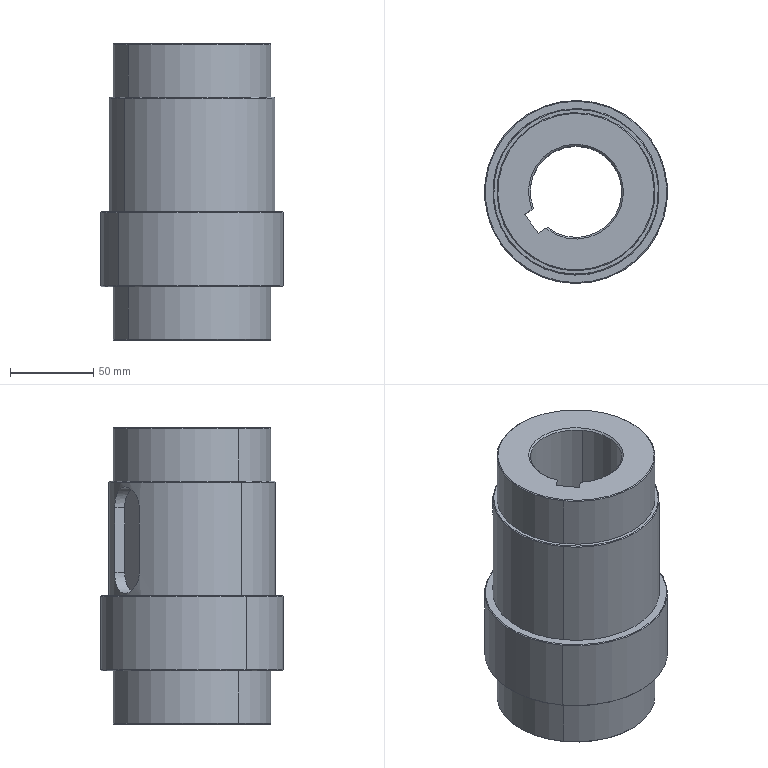Part | SolidWorks | features BaseBody 1 | 1 solid | 37 faces | box 110 x 110 x 178 mm | volume 973022 mm3 | cylinder 13 | cone 13 | plane 11 | commonest cylinder face diameters 95 x4 25 x3 55 x2 100 x2 110 x2
STEP:
#1=CARTESIAN_POINT('',(507.1,275.211,-200.693));
#2=VERTEX_POINT('',#1);
#3=CARTESIAN_POINT('',(497.014,267.828,-188.193));
#4=VERTEX_POINT('',#3);
#5=CARTESIAN_POINT('',(497.014,267.828,-200.693));
#6=DIRECTION('',(0.5907,-0.8069,0.));
#7=DIRECTION('',(0.,0.,-1.));
#8=AXIS2_PLACEMENT_3D('',#5,#6,#7);
#9=CIRCLE('',#8,12.5);
#10=EDGE_CURVE('',#2,#4,#9,.T.);
#11=ORIENTED_EDGE('',*,*,#10,.T.);
#12=CARTESIAN_POINT('',(491.698,275.09,-188.193));
#13=VERTEX_POINT('',#12);
#14=CARTESIAN_POINT('',(497.014,267.828,-188.193));
#15=DIRECTION('',(-0.5907,0.8069,0.));
#16=VECTOR('',#15,1000.);
#17=LINE('',#14,#16);
#18=EDGE_CURVE('',#4,#13,#17,.T.);
#19=ORIENTED_EDGE('',*,*,#18,.T.);
#20=CARTESIAN_POINT('',(502.722,281.192,-200.693));
#21=VERTEX_POINT('',#20);
#22=CARTESIAN_POINT('',(502.722,281.192,-200.693));
#23=CARTESIAN_POINT('',(502.722,281.192,-199.863));
#24=CARTESIAN_POINT('',(502.643,281.161,-199.048));
#25=CARTESIAN_POINT('',(502.414,281.068,-197.846));
#26=CARTESIAN_POINT('',(502.319,281.03,-197.449));
#27=CARTESIAN_POINT('',(502.091,280.936,-196.662));
#28=CARTESIAN_POINT('',(501.958,280.88,-196.272));
#29=CARTESIAN_POINT('',(501.511,280.692,-195.137));
#30=CARTESIAN_POINT('',(501.149,280.536,-194.42));
#31=CARTESIAN_POINT('',(500.514,280.251,-193.403));
#32=CARTESIAN_POINT('',(500.286,280.146,-193.072));
#33=CARTESIAN_POINT('',(499.805,279.922,-192.439));
#34=CARTESIAN_POINT('',(499.554,279.802,-192.137));
#35=CARTESIAN_POINT('',(498.767,279.418,-191.276));
#36=CARTESIAN_POINT('',(498.2,279.13,-190.76));
#37=CARTESIAN_POINT('',(497.289,278.64,-190.075));
#38=CARTESIAN_POINT('',(496.977,278.469,-189.863));
#39=CARTESIAN_POINT('',(496.346,278.113,-189.478));
#40=CARTESIAN_POINT('',(496.025,277.928,-189.304));
#41=CARTESIAN_POINT('',(495.376,277.542,-188.992));
#42=CARTESIAN_POINT('',(495.047,277.342,-188.854));
#43=CARTESIAN_POINT('',(494.38,276.924,-188.615));
#44=CARTESIAN_POINT('',(494.04,276.706,-188.514));
#45=CARTESIAN_POINT('',(493.027,276.038,-188.273));
#46=CARTESIAN_POINT('',(492.359,275.574,-188.193));
#47=CARTESIAN_POINT('',(491.698,275.09,-188.193));
#48=B_SPLINE_CURVE_WITH_KNOTS('',3,(#22,#23,#24,#25,#26,#27,#28,#29,#30,#31,#32,#33,#34,#35,#36,#37,#38,#39,#40,#41,#42,#43,#44,#45,#46,#47),.UNSPECIFIED.,.F.,.F.,(4,2,2,2,2,2,2,2,2,2,2,2,4),(0.,0.002453,0.003679,0.004906,0.007359,0.008585,0.009812,0.01226,0.01349,0.01472,0.01594,0.01717,0.01962),.UNSPECIFIED.);
#49=EDGE_CURVE('',#21,#13,#48,.T.);
#50=ORIENTED_EDGE('',*,*,#49,.F.);
#51=CARTESIAN_POINT('',(507.1,275.211,-200.693));
#52=DIRECTION('',(-0.5907,0.8069,0.));
#53=VECTOR('',#52,1000.);
#54=LINE('',#51,#53);
#55=EDGE_CURVE('',#2,#21,#54,.T.);
#56=ORIENTED_EDGE('',*,*,#55,.F.);
#57=EDGE_LOOP('',(#11,#19,#50,#56));
#58=FACE_OUTER_BOUND('',#57,.T.);
#59=CARTESIAN_POINT('',(497.014,267.828,-200.693));
#60=DIRECTION('',(-0.5907,0.8069,0.));
#61=DIRECTION('',(0.,0.,1.));
#62=AXIS2_PLACEMENT_3D('',#59,#60,#61);
#63=CYLINDRICAL_SURFACE('',#62,12.5);
#64=ADVANCED_FACE('',(#58),#63,.F.);
#65=CARTESIAN_POINT('',(559.156,262.505,-330.693));
#66=VERTEX_POINT('',#65);
#67=CARTESIAN_POINT('',(483.305,206.983,-330.693));
#68=VERTEX_POINT('',#67);
#69=CARTESIAN_POINT('',(521.231,234.744,-330.693));
#70=DIRECTION('',(0.,0.,-1.));
#71=DIRECTION('',(0.8069,0.5907,0.));
#72=AXIS2_PLACEMENT_3D('',#69,#70,#71);
#73=CIRCLE('',#72,47.);
#74=EDGE_CURVE('',#66,#68,#73,.T.);
#75=ORIENTED_EDGE('',*,*,#74,.F.);
#76=CARTESIAN_POINT('',(559.559,262.8,-330.193));
#77=VERTEX_POINT('',#76);
#78=CARTESIAN_POINT('',(559.156,262.505,-330.693));
#79=DIRECTION('',(0.5706,0.4177,0.7071));
#80=VECTOR('',#79,1000.);
#81=LINE('',#78,#80);
#82=EDGE_CURVE('',#66,#77,#81,.T.);
#83=ORIENTED_EDGE('',*,*,#82,.T.);
#84=CARTESIAN_POINT('',(482.902,206.688,-330.193));
#85=VERTEX_POINT('',#84);
#86=CARTESIAN_POINT('',(521.231,234.744,-330.193));
#87=DIRECTION('',(0.,0.,1.));
#88=DIRECTION('',(0.8069,0.5907,0.));
#89=AXIS2_PLACEMENT_3D('',#86,#87,#88);
#90=CIRCLE('',#89,47.5);
#91=EDGE_CURVE('',#85,#77,#90,.T.);
#92=ORIENTED_EDGE('',*,*,#91,.F.);
#93=CARTESIAN_POINT('',(483.305,206.983,-330.693));
#94=DIRECTION('',(-0.5706,-0.4177,0.7071));
#95=VECTOR('',#94,1000.);
#96=LINE('',#93,#95);
#97=EDGE_CURVE('',#68,#85,#96,.T.);
#98=ORIENTED_EDGE('',*,*,#97,.F.);
#99=EDGE_LOOP('',(#75,#83,#92,#98));
#100=FACE_OUTER_BOUND('',#99,.T.);
#101=CARTESIAN_POINT('',(521.231,234.744,-330.693));
#102=DIRECTION('',(0.,0.,1.));
#103=DIRECTION('',(-0.8069,-0.5907,0.));
#104=AXIS2_PLACEMENT_3D('',#101,#102,#103);
#105=CONICAL_SURFACE('',#104,47.,0.7854);
#106=ADVANCED_FACE('',(#100),#105,.T.);
#107=CARTESIAN_POINT('',(565.208,266.935,-298.693));
#108=VERTEX_POINT('',#107);
#109=CARTESIAN_POINT('',(477.253,202.553,-298.693));
#110=VERTEX_POINT('',#109);
#111=CARTESIAN_POINT('',(521.231,234.744,-298.693));
#112=DIRECTION('',(0.,0.,-1.));
#113=DIRECTION('',(0.8069,0.5907,0.));
#114=AXIS2_PLACEMENT_3D('',#111,#112,#113);
#115=CIRCLE('',#114,54.5);
#116=EDGE_CURVE('',#108,#110,#115,.T.);
#117=ORIENTED_EDGE('',*,*,#116,.F.);
#118=CARTESIAN_POINT('',(565.611,267.23,-298.193));
#119=VERTEX_POINT('',#118);
#120=CARTESIAN_POINT('',(565.208,266.935,-298.693));
#121=DIRECTION('',(0.5706,0.4177,0.7071));
#122=VECTOR('',#121,1000.);
#123=LINE('',#120,#122);
#124=EDGE_CURVE('',#108,#119,#123,.T.);
#125=ORIENTED_EDGE('',*,*,#124,.T.);
#126=CARTESIAN_POINT('',(476.85,202.258,-298.193));
#127=VERTEX_POINT('',#126);
#128=CARTESIAN_POINT('',(521.231,234.744,-298.193));
#129=DIRECTION('',(0.,0.,1.));
#130=DIRECTION('',(0.8069,0.5907,0.));
#131=AXIS2_PLACEMENT_3D('',#128,#129,#130);
#132=CIRCLE('',#131,55.);
#133=EDGE_CURVE('',#127,#119,#132,.T.);
#134=ORIENTED_EDGE('',*,*,#133,.F.);
#135=CARTESIAN_POINT('',(477.253,202.553,-298.693));
#136=DIRECTION('',(-0.5706,-0.4177,0.7071));
#137=VECTOR('',#136,1000.);
#138=LINE('',#135,#137);
#139=EDGE_CURVE('',#110,#127,#138,.T.);
#140=ORIENTED_EDGE('',*,*,#139,.F.);
#141=EDGE_LOOP('',(#117,#125,#134,#140));
#142=FACE_OUTER_BOUND('',#141,.T.);
#143=CARTESIAN_POINT('',(521.231,234.744,-298.693));
#144=DIRECTION('',(0.,0.,1.));
#145=DIRECTION('',(-0.8069,-0.5907,0.));
#146=AXIS2_PLACEMENT_3D('',#143,#144,#145);
#147=CONICAL_SURFACE('',#146,54.5,0.7854);
#148=ADVANCED_FACE('',(#142),#147,.T.);
#149=CARTESIAN_POINT('',(477.253,202.553,-253.693));
#150=VERTEX_POINT('',#149);
#151=CARTESIAN_POINT('',(565.208,266.935,-253.693));
#152=VERTEX_POINT('',#151);
#153=CARTESIAN_POINT('',(521.231,234.744,-253.693));
#154=DIRECTION('',(0.,0.,1.));
#155=DIRECTION('',(-0.8069,-0.5907,0.));
#156=AXIS2_PLACEMENT_3D('',#153,#154,#155);
#157=CIRCLE('',#156,54.5);
#158=EDGE_CURVE('',#150,#152,#157,.T.);
#159=ORIENTED_EDGE('',*,*,#158,.F.);
#160=CARTESIAN_POINT('',(476.85,202.258,-254.193));
#161=VERTEX_POINT('',#160);
#162=CARTESIAN_POINT('',(477.253,202.553,-253.693));
#163=DIRECTION('',(-0.5706,-0.4177,-0.7071));
#164=VECTOR('',#163,1000.);
#165=LINE('',#162,#164);
#166=EDGE_CURVE('',#150,#161,#165,.T.);
#167=ORIENTED_EDGE('',*,*,#166,.T.);
#168=CARTESIAN_POINT('',(565.611,267.23,-254.193));
#169=VERTEX_POINT('',#168);
#170=CARTESIAN_POINT('',(521.231,234.744,-254.193));
#171=DIRECTION('',(0.,0.,-1.));
#172=DIRECTION('',(-0.8069,-0.5907,0.));
#173=AXIS2_PLACEMENT_3D('',#170,#171,#172);
#174=CIRCLE('',#173,55.);
#175=EDGE_CURVE('',#169,#161,#174,.T.);
#176=ORIENTED_EDGE('',*,*,#175,.F.);
#177=CARTESIAN_POINT('',(565.208,266.935,-253.693));
#178=DIRECTION('',(0.5706,0.4177,-0.7071));
#179=VECTOR('',#178,1000.);
#180=LINE('',#177,#179);
#181=EDGE_CURVE('',#152,#169,#180,.T.);
#182=ORIENTED_EDGE('',*,*,#181,.F.);
#183=EDGE_LOOP('',(#159,#167,#176,#182));
#184=FACE_OUTER_BOUND('',#183,.T.);
#185=CARTESIAN_POINT('',(521.231,234.744,-253.693));
#186=DIRECTION('',(0.,0.,-1.));
#187=DIRECTION('',(0.8069,0.5907,0.));
#188=AXIS2_PLACEMENT_3D('',#185,#186,#187);
#189=CONICAL_SURFACE('',#188,54.5,0.7854);
#190=ADVANCED_FACE('',(#184),#189,.T.);
#191=CARTESIAN_POINT('',(481.288,205.506,-184.693));
#192=VERTEX_POINT('',#191);
#193=CARTESIAN_POINT('',(561.173,263.982,-184.693));
#194=VERTEX_POINT('',#193);
#195=CARTESIAN_POINT('',(521.231,234.744,-184.693));
#196=DIRECTION('',(0.,0.,1.));
#197=DIRECTION('',(0.8069,0.5907,0.));
#198=AXIS2_PLACEMENT_3D('',#195,#196,#197);
#199=CIRCLE('',#198,49.5);
#200=EDGE_CURVE('',#192,#194,#199,.T.);
#201=ORIENTED_EDGE('',*,*,#200,.F.);
#202=CARTESIAN_POINT('',(480.885,205.211,-185.193));
#203=VERTEX_POINT('',#202);
#204=CARTESIAN_POINT('',(481.288,205.506,-184.693));
#205=DIRECTION('',(-0.5706,-0.4177,-0.7071));
#206=VECTOR('',#205,1000.);
#207=LINE('',#204,#206);
#208=EDGE_CURVE('',#192,#203,#207,.T.);
#209=ORIENTED_EDGE('',*,*,#208,.T.);
#210=CARTESIAN_POINT('',(561.577,264.277,-185.193));
#211=VERTEX_POINT('',#210);
#212=CARTESIAN_POINT('',(521.231,234.744,-185.193));
#213=DIRECTION('',(0.,0.,-1.));
#214=DIRECTION('',(0.8069,0.5907,0.));
#215=AXIS2_PLACEMENT_3D('',#212,#213,#214);
#216=CIRCLE('',#215,50.);
#217=EDGE_CURVE('',#211,#203,#216,.T.);
#218=ORIENTED_EDGE('',*,*,#217,.F.);
#219=CARTESIAN_POINT('',(561.173,263.982,-184.693));
#220=DIRECTION('',(0.5706,0.4177,-0.7071));
#221=VECTOR('',#220,1000.);
#222=LINE('',#219,#221);
#223=EDGE_CURVE('',#194,#211,#222,.T.);
#224=ORIENTED_EDGE('',*,*,#223,.F.);
#225=EDGE_LOOP('',(#201,#209,#218,#224));
#226=FACE_OUTER_BOUND('',#225,.T.);
#227=CARTESIAN_POINT('',(521.231,234.744,-184.693));
#228=DIRECTION('',(0.,0.,-1.));
#229=DIRECTION('',(0.8069,0.5907,0.));
#230=AXIS2_PLACEMENT_3D('',#227,#228,#229);
#231=CONICAL_SURFACE('',#230,49.5,0.7854);
#232=ADVANCED_FACE('',(#226),#231,.T.);
#233=CARTESIAN_POINT('',(483.305,206.983,-152.693));
#234=VERTEX_POINT('',#233);
#235=CARTESIAN_POINT('',(559.156,262.505,-152.693));
#236=VERTEX_POINT('',#235);
#237=CARTESIAN_POINT('',(521.231,234.744,-152.693));
#238=DIRECTION('',(0.,0.,1.));
#239=DIRECTION('',(-0.8069,-0.5907,0.));
#240=AXIS2_PLACEMENT_3D('',#237,#238,#239);
#241=CIRCLE('',#240,47.);
#242=EDGE_CURVE('',#234,#236,#241,.T.);
#243=ORIENTED_EDGE('',*,*,#242,.F.);
#244=CARTESIAN_POINT('',(482.902,206.688,-153.193));
#245=VERTEX_POINT('',#244);
#246=CARTESIAN_POINT('',(483.305,206.983,-152.693));
#247=DIRECTION('',(-0.5706,-0.4177,-0.7071));
#248=VECTOR('',#247,1000.);
#249=LINE('',#246,#248);
#250=EDGE_CURVE('',#234,#245,#249,.T.);
#251=ORIENTED_EDGE('',*,*,#250,.T.);
#252=CARTESIAN_POINT('',(559.559,262.8,-153.193));
#253=VERTEX_POINT('',#252);
#254=CARTESIAN_POINT('',(521.231,234.744,-153.193));
#255=DIRECTION('',(0.,0.,-1.));
#256=DIRECTION('',(-0.8069,-0.5907,0.));
#257=AXIS2_PLACEMENT_3D('',#254,#255,#256);
#258=CIRCLE('',#257,47.5);
#259=EDGE_CURVE('',#253,#245,#258,.T.);
#260=ORIENTED_EDGE('',*,*,#259,.F.);
#261=CARTESIAN_POINT('',(559.156,262.505,-152.693));
#262=DIRECTION('',(0.5706,0.4177,-0.7071));
#263=VECTOR('',#262,1000.);
#264=LINE('',#261,#263);
#265=EDGE_CURVE('',#236,#253,#264,.T.);
#266=ORIENTED_EDGE('',*,*,#265,.F.);
#267=EDGE_LOOP('',(#243,#251,#260,#266));
#268=FACE_OUTER_BOUND('',#267,.T.);
#269=CARTESIAN_POINT('',(521.231,234.744,-152.693));
#270=DIRECTION('',(0.,0.,-1.));
#271=DIRECTION('',(0.8069,0.5907,0.));
#272=AXIS2_PLACEMENT_3D('',#269,#270,#271);
#273=CONICAL_SURFACE('',#272,47.,0.7854);
#274=ADVANCED_FACE('',(#268),#273,.T.);
#275=CARTESIAN_POINT('',(543.421,250.987,-329.693));
#276=VERTEX_POINT('',#275);
#277=CARTESIAN_POINT('',(503.906,213.387,-329.693));
#278=VERTEX_POINT('',#277);
#279=CARTESIAN_POINT('',(521.231,234.744,-329.693));
#280=DIRECTION('',(0.,0.,-1.));
#281=DIRECTION('',(0.8069,0.5907,0.));
#282=AXIS2_PLACEMENT_3D('',#279,#280,#281);
#283=CIRCLE('',#282,27.5);
#284=EDGE_CURVE('',#276,#278,#283,.T.);
#285=ORIENTED_EDGE('',*,*,#284,.F.);
#286=CARTESIAN_POINT('',(544.228,251.578,-330.693));
#287=VERTEX_POINT('',#286);
#288=CARTESIAN_POINT('',(543.421,250.987,-329.693));
#289=DIRECTION('',(0.5706,0.4177,-0.7071));
#290=VECTOR('',#289,1000.);
#291=LINE('',#288,#290);
#292=EDGE_CURVE('',#276,#287,#291,.T.);
#293=ORIENTED_EDGE('',*,*,#292,.T.);
#294=CARTESIAN_POINT('',(503.072,212.777,-330.693));
#295=VERTEX_POINT('',#294);
#296=CARTESIAN_POINT('',(521.231,234.744,-330.693));
#297=DIRECTION('',(0.,0.,1.));
#298=DIRECTION('',(0.8069,0.5907,0.));
#299=AXIS2_PLACEMENT_3D('',#296,#297,#298);
#300=CIRCLE('',#299,28.5);
#301=EDGE_CURVE('',#295,#287,#300,.T.);
#302=ORIENTED_EDGE('',*,*,#301,.F.);
#303=CARTESIAN_POINT('',(503.906,213.387,-329.693));
#304=CARTESIAN_POINT('',(503.628,213.184,-330.026));
#305=CARTESIAN_POINT('',(503.35,212.981,-330.359));
#306=CARTESIAN_POINT('',(503.072,212.777,-330.693));
#307=B_SPLINE_CURVE_WITH_KNOTS('',3,(#303,#304,#305,#306),.UNSPECIFIED.,.F.,.F.,(4,4),(0.006995,0.008432),.UNSPECIFIED.);
#308=EDGE_CURVE('',#278,#295,#307,.T.);
#309=ORIENTED_EDGE('',*,*,#308,.F.);
#310=EDGE_LOOP('',(#285,#293,#302,#309));
#311=FACE_OUTER_BOUND('',#310,.T.);
#312=CARTESIAN_POINT('',(521.231,234.744,-329.693));
#313=DIRECTION('',(0.,0.,-1.));
#314=DIRECTION('',(0.8069,0.5907,0.));
#315=AXIS2_PLACEMENT_3D('',#312,#313,#314);
#316=CONICAL_SURFACE('',#315,27.5,0.7854);
#317=ADVANCED_FACE('',(#311),#316,.F.);
#318=CARTESIAN_POINT('',(503.906,213.387,-153.693));
#319=VERTEX_POINT('',#318);
#320=CARTESIAN_POINT('',(543.421,250.987,-153.693));
#321=VERTEX_POINT('',#320);
#322=CARTESIAN_POINT('',(521.231,234.744,-153.693));
#323=DIRECTION('',(0.,0.,1.));
#324=DIRECTION('',(-0.8069,-0.5907,0.));
#325=AXIS2_PLACEMENT_3D('',#322,#323,#324);
#326=CIRCLE('',#325,27.5);
#327=EDGE_CURVE('',#319,#321,#326,.T.);
#328=ORIENTED_EDGE('',*,*,#327,.T.);
#329=CARTESIAN_POINT('',(543.421,250.987,-152.693));
#330=DIRECTION('',(0.,0.,-1.));
#331=VECTOR('',#330,1000.);
#332=LINE('',#329,#331);
#333=EDGE_CURVE('',#321,#276,#332,.T.);
#334=ORIENTED_EDGE('',*,*,#333,.T.);
#335=ORIENTED_EDGE('',*,*,#284,.T.);
#336=CARTESIAN_POINT('',(503.906,213.387,-152.693));
#337=DIRECTION('',(0.,0.,1.));
#338=VECTOR('',#337,1000.);
#339=LINE('',#336,#338);
#340=EDGE_CURVE('',#278,#319,#339,.T.);
#341=ORIENTED_EDGE('',*,*,#340,.T.);
#342=EDGE_LOOP('',(#328,#334,#335,#341));
#343=FACE_OUTER_BOUND('',#342,.T.);
#344=CARTESIAN_POINT('',(521.231,234.744,-152.693));
#345=DIRECTION('',(0.,0.,-1.));
#346=DIRECTION('',(0.8069,0.5907,0.));
#347=AXIS2_PLACEMENT_3D('',#344,#345,#346);
#348=CYLINDRICAL_SURFACE('',#347,27.5);
#349=ADVANCED_FACE('',(#343),#348,.F.);
#350=ORIENTED_EDGE('',*,*,#259,.T.);
#351=CARTESIAN_POINT('',(482.902,206.688,-184.693));
#352=VERTEX_POINT('',#351);
#353=CARTESIAN_POINT('',(482.902,206.688,-152.693));
#354=DIRECTION('',(0.,0.,-1.));
#355=VECTOR('',#354,1000.);
#356=LINE('',#353,#355);
#357=EDGE_CURVE('',#245,#352,#356,.T.);
#358=ORIENTED_EDGE('',*,*,#357,.T.);
#359=CARTESIAN_POINT('',(559.559,262.8,-184.693));
#360=VERTEX_POINT('',#359);
#361=CARTESIAN_POINT('',(521.231,234.744,-184.693));
#362=DIRECTION('',(0.,0.,1.));
#363=DIRECTION('',(0.8069,0.5907,0.));
#364=AXIS2_PLACEMENT_3D('',#361,#362,#363);
#365=CIRCLE('',#364,47.5);
#366=EDGE_CURVE('',#352,#360,#365,.T.);
#367=ORIENTED_EDGE('',*,*,#366,.T.);
#368=CARTESIAN_POINT('',(559.559,262.8,-152.693));
#369=DIRECTION('',(0.,0.,-1.));
#370=VECTOR('',#369,1000.);
#371=LINE('',#368,#370);
#372=EDGE_CURVE('',#253,#360,#371,.T.);
#373=ORIENTED_EDGE('',*,*,#372,.F.);
#374=EDGE_LOOP('',(#350,#358,#367,#373));
#375=FACE_OUTER_BOUND('',#374,.T.);
#376=CARTESIAN_POINT('',(521.231,234.744,-152.693));
#377=DIRECTION('',(0.,0.,-1.));
#378=DIRECTION('',(0.8069,0.5907,0.));
#379=AXIS2_PLACEMENT_3D('',#376,#377,#378);
#380=CYLINDRICAL_SURFACE('',#379,47.5);
#381=ADVANCED_FACE('',(#375),#380,.T.);
#382=ORIENTED_EDGE('',*,*,#91,.T.);
#383=CARTESIAN_POINT('',(559.559,262.8,-298.693));
#384=VERTEX_POINT('',#383);
#385=CARTESIAN_POINT('',(559.559,262.8,-330.693));
#386=DIRECTION('',(0.,0.,1.));
#387=VECTOR('',#386,1000.);
#388=LINE('',#385,#387);
#389=EDGE_CURVE('',#77,#384,#388,.T.);
#390=ORIENTED_EDGE('',*,*,#389,.T.);
#391=CARTESIAN_POINT('',(482.902,206.688,-298.693));
#392=VERTEX_POINT('',#391);
#393=CARTESIAN_POINT('',(521.231,234.744,-298.693));
#394=DIRECTION('',(0.,0.,-1.));
#395=DIRECTION('',(0.8069,0.5907,0.));
#396=AXIS2_PLACEMENT_3D('',#393,#394,#395);
#397=CIRCLE('',#396,47.5);
#398=EDGE_CURVE('',#384,#392,#397,.T.);
#399=ORIENTED_EDGE('',*,*,#398,.T.);
#400=CARTESIAN_POINT('',(482.902,206.688,-330.693));
#401=DIRECTION('',(0.,0.,1.));
#402=VECTOR('',#401,1000.);
#403=LINE('',#400,#402);
#404=EDGE_CURVE('',#85,#392,#403,.T.);
#405=ORIENTED_EDGE('',*,*,#404,.F.);
#406=EDGE_LOOP('',(#382,#390,#399,#405));
#407=FACE_OUTER_BOUND('',#406,.T.);
#408=CARTESIAN_POINT('',(521.231,234.744,-330.693));
#409=DIRECTION('',(0.,0.,1.));
#410=DIRECTION('',(-0.8069,-0.5907,0.));
#411=AXIS2_PLACEMENT_3D('',#408,#409,#410);
#412=CYLINDRICAL_SURFACE('',#411,47.5);
#413=ADVANCED_FACE('',(#407),#412,.T.);
#414=ORIENTED_EDGE('',*,*,#133,.T.);
#415=CARTESIAN_POINT('',(565.611,267.23,-298.693));
#416=DIRECTION('',(0.,0.,1.));
#417=VECTOR('',#416,1000.);
#418=LINE('',#415,#417);
#419=EDGE_CURVE('',#119,#169,#418,.T.);
#420=ORIENTED_EDGE('',*,*,#419,.T.);
#421=ORIENTED_EDGE('',*,*,#175,.T.);
#422=CARTESIAN_POINT('',(476.85,202.258,-298.693));
#423=DIRECTION('',(0.,0.,1.));
#424=VECTOR('',#423,1000.);
#425=LINE('',#422,#424);
#426=EDGE_CURVE('',#127,#161,#425,.T.);
#427=ORIENTED_EDGE('',*,*,#426,.F.);
#428=EDGE_LOOP('',(#414,#420,#421,#427));
#429=FACE_OUTER_BOUND('',#428,.T.);
#430=CARTESIAN_POINT('',(521.231,234.744,-298.693));
#431=DIRECTION('',(0.,0.,1.));
#432=DIRECTION('',(-0.8069,-0.5907,0.));
#433=AXIS2_PLACEMENT_3D('',#430,#431,#432);
#434=CYLINDRICAL_SURFACE('',#433,55.);
#435=ADVANCED_FACE('',(#429),#434,.T.);
#436=CARTESIAN_POINT('',(480.885,205.211,-253.693));
#437=VERTEX_POINT('',#436);
#438=CARTESIAN_POINT('',(561.577,264.277,-253.693));
#439=VERTEX_POINT('',#438);
#440=CARTESIAN_POINT('',(521.231,234.744,-253.693));
#441=DIRECTION('',(0.,0.,1.));
#442=DIRECTION('',(-0.8069,-0.5907,0.));
#443=AXIS2_PLACEMENT_3D('',#440,#441,#442);
#444=CIRCLE('',#443,50.);
#445=EDGE_CURVE('',#437,#439,#444,.T.);
#446=ORIENTED_EDGE('',*,*,#445,.T.);
#447=CARTESIAN_POINT('',(561.577,264.277,-253.693));
#448=DIRECTION('',(0.,0.,1.));
#449=VECTOR('',#448,1000.);
#450=LINE('',#447,#449);
#451=EDGE_CURVE('',#439,#211,#450,.T.);
#452=ORIENTED_EDGE('',*,*,#451,.T.);
#453=ORIENTED_EDGE('',*,*,#217,.T.);
#454=CARTESIAN_POINT('',(480.885,205.211,-253.693));
#455=DIRECTION('',(0.,0.,1.));
#456=VECTOR('',#455,1000.);
#457=LINE('',#454,#456);
#458=EDGE_CURVE('',#437,#203,#457,.T.);
#459=ORIENTED_EDGE('',*,*,#458,.F.);
#460=EDGE_LOOP('',(#446,#452,#453,#459));
#461=FACE_OUTER_BOUND('',#460,.T.);
#462=CARTESIAN_POINT('',(521.231,234.744,-253.693));
#463=DIRECTION('',(0.,0.,1.));
#464=DIRECTION('',(-0.8069,-0.5907,0.));
#465=AXIS2_PLACEMENT_3D('',#462,#463,#464);
#466=CYLINDRICAL_SURFACE('',#465,50.);
#467=ADVANCED_FACE('',(#461),#466,.T.);
#468=ORIENTED_EDGE('',*,*,#451,.F.);
#469=CARTESIAN_POINT('',(521.231,234.744,-253.693));
#470=DIRECTION('',(0.,0.,1.));
#471=DIRECTION('',(-0.8069,-0.5907,0.));
#472=AXIS2_PLACEMENT_3D('',#469,#470,#471);
#473=CIRCLE('',#472,50.);
#474=EDGE_CURVE('',#439,#437,#473,.T.);
#475=ORIENTED_EDGE('',*,*,#474,.T.);
#476=ORIENTED_EDGE('',*,*,#458,.T.);
#477=CARTESIAN_POINT('',(521.231,234.744,-185.193));
#478=DIRECTION('',(0.,0.,-1.));
#479=DIRECTION('',(0.8069,0.5907,0.));
#480=AXIS2_PLACEMENT_3D('',#477,#478,#479);
#481=CIRCLE('',#480,50.);
#482=EDGE_CURVE('',#203,#211,#481,.T.);
#483=ORIENTED_EDGE('',*,*,#482,.T.);
#484=EDGE_LOOP('',(#468,#475,#476,#483));
#485=FACE_OUTER_BOUND('',#484,.T.);
#486=CARTESIAN_POINT('',(482.549,266.426,-200.693));
#487=VERTEX_POINT('',#486);
#488=CARTESIAN_POINT('',(482.549,266.426,-239.693));
#489=VERTEX_POINT('',#488);
#490=CARTESIAN_POINT('',(482.549,266.426,-253.693));
#491=DIRECTION('',(0.,0.,-1.));
#492=VECTOR('',#491,1000.);
#493=LINE('',#490,#492);
#494=EDGE_CURVE('',#487,#489,#493,.T.);
#495=ORIENTED_EDGE('',*,*,#494,.T.);
#496=CARTESIAN_POINT('',(502.722,281.192,-239.693));
#497=VERTEX_POINT('',#496);
#498=CARTESIAN_POINT('',(482.549,266.426,-239.693));
#499=CARTESIAN_POINT('',(482.549,266.426,-240.522));
#500=CARTESIAN_POINT('',(482.602,266.491,-241.337));
#501=CARTESIAN_POINT('',(482.76,266.681,-242.538));
#502=CARTESIAN_POINT('',(482.825,266.76,-242.935));
#503=CARTESIAN_POINT('',(482.984,266.949,-243.722));
#504=CARTESIAN_POINT('',(483.077,267.059,-244.112));
#505=CARTESIAN_POINT('',(483.391,267.428,-245.246));
#506=CARTESIAN_POINT('',(483.649,267.726,-245.962));
#507=CARTESIAN_POINT('',(484.112,268.244,-246.979));
#508=CARTESIAN_POINT('',(484.28,268.43,-247.31));
#509=CARTESIAN_POINT('',(484.639,268.819,-247.943));
#510=CARTESIAN_POINT('',(484.829,269.023,-248.245));
#511=CARTESIAN_POINT('',(485.433,269.656,-249.106));
#512=CARTESIAN_POINT('',(485.878,270.109,-249.622));
#513=CARTESIAN_POINT('',(486.619,270.83,-250.307));
#514=CARTESIAN_POINT('',(486.877,271.075,-250.519));
#515=CARTESIAN_POINT('',(487.406,271.568,-250.904));
#516=CARTESIAN_POINT('',(487.679,271.817,-251.078));
#517=CARTESIAN_POINT('',(488.243,272.32,-251.391));
#518=CARTESIAN_POINT('',(488.533,272.573,-251.529));
#519=CARTESIAN_POINT('',(489.132,273.082,-251.768));
#520=CARTESIAN_POINT('',(489.442,273.34,-251.87));
#521=CARTESIAN_POINT('',(490.384,274.103,-252.112));
#522=CARTESIAN_POINT('',(491.028,274.6,-252.192));
#523=CARTESIAN_POINT('',(492.349,275.567,-252.194));
#524=CARTESIAN_POINT('',(493.033,276.042,-252.112));
#525=CARTESIAN_POINT('',(494.375,276.927,-251.792));
#526=CARTESIAN_POINT('',(495.039,277.342,-251.555));
#527=CARTESIAN_POINT('',(496.022,277.926,-251.084));
#528=CARTESIAN_POINT('',(496.348,278.114,-250.907));
#529=CARTESIAN_POINT('',(496.98,278.471,-250.521));
#530=CARTESIAN_POINT('',(497.288,278.64,-250.311));
#531=CARTESIAN_POINT('',(497.889,278.963,-249.86));
#532=CARTESIAN_POINT('',(498.182,279.116,-249.618));
#533=CARTESIAN_POINT('',(498.75,279.406,-249.101));
#534=CARTESIAN_POINT('',(499.027,279.545,-248.825));
#535=CARTESIAN_POINT('',(499.82,279.932,-247.957));
#536=CARTESIAN_POINT('',(500.297,280.153,-247.33));
#537=CARTESIAN_POINT('',(500.93,280.438,-246.317));
#538=CARTESIAN_POINT('',(501.127,280.525,-245.968));
#539=CARTESIAN_POINT('',(501.493,280.684,-245.243));
#540=CARTESIAN_POINT('',(501.66,280.755,-244.871));
#541=CARTESIAN_POINT('',(502.105,280.943,-243.74));
#542=CARTESIAN_POINT('',(502.333,281.035,-242.961));
#543=CARTESIAN_POINT('',(502.565,281.129,-241.754));
#544=CARTESIAN_POINT('',(502.624,281.153,-241.344));
#545=CARTESIAN_POINT('',(502.702,281.184,-240.521));
#546=CARTESIAN_POINT('',(502.722,281.192,-240.108));
#547=CARTESIAN_POINT('',(502.722,281.192,-239.693));
#548=B_SPLINE_CURVE_WITH_KNOTS('',3,(#498,#499,#500,#501,#502,#503,#504,#505,#506,#507,#508,#509,#510,#511,#512,#513,#514,#515,#516,#517,#518,#519,#520,#521,#522,#523,#524,#525,#526,#527,#528,#529,#530,#531,#532,#533,#534,#535,#536,#537,#538,#539,#540,#541,#542,#543,#544,#545,#546,#547),.UNSPECIFIED.,.F.,.F.,(4,2,2,2,2,2,2,2,2,2,2,2,2,2,2,2,2,2,2,2,2,2,2,2,4),(0.,0.002452,0.003677,0.004903,0.007355,0.00858,0.009806,0.01226,0.01348,0.01471,0.01593,0.01716,0.01961,0.02206,0.02452,0.02574,0.02697,0.02819,0.02942,0.03187,0.0331,0.03432,0.03677,0.038,0.03922),.UNSPECIFIED.);
#549=EDGE_CURVE('',#489,#497,#548,.T.);
#550=ORIENTED_EDGE('',*,*,#549,.T.);
#551=CARTESIAN_POINT('',(502.722,281.192,-253.693));
#552=DIRECTION('',(0.,0.,1.));
#553=VECTOR('',#552,1000.);
#554=LINE('',#551,#553);
#555=EDGE_CURVE('',#497,#21,#554,.T.);
#556=ORIENTED_EDGE('',*,*,#555,.T.);
#557=ORIENTED_EDGE('',*,*,#49,.T.);
#558=CARTESIAN_POINT('',(491.698,275.09,-188.193));
#559=CARTESIAN_POINT('',(491.037,274.607,-188.193));
#560=CARTESIAN_POINT('',(490.379,274.099,-188.275));
#561=CARTESIAN_POINT('',(489.131,273.088,-188.596));
#562=CARTESIAN_POINT('',(488.535,272.58,-188.833));
#563=CARTESIAN_POINT('',(487.682,271.82,-189.306));
#564=CARTESIAN_POINT('',(487.405,271.567,-189.483));
#565=CARTESIAN_POINT('',(486.874,271.072,-189.869));
#566=CARTESIAN_POINT('',(486.62,270.83,-190.078));
#567=CARTESIAN_POINT('',(486.131,270.355,-190.53));
#568=CARTESIAN_POINT('',(485.897,270.122,-190.772));
#569=CARTESIAN_POINT('',(485.449,269.669,-191.289));
#570=CARTESIAN_POINT('',(485.233,269.447,-191.565));
#571=CARTESIAN_POINT('',(484.625,268.808,-192.433));
#572=CARTESIAN_POINT('',(484.271,268.421,-193.06));
#573=CARTESIAN_POINT('',(483.808,267.905,-194.072));
#574=CARTESIAN_POINT('',(483.666,267.743,-194.422));
#575=CARTESIAN_POINT('',(483.404,267.443,-195.146));
#576=CARTESIAN_POINT('',(483.286,267.305,-195.518));
#577=CARTESIAN_POINT('',(482.973,266.938,-196.648));
#578=CARTESIAN_POINT('',(482.816,266.749,-197.427));
#579=CARTESIAN_POINT('',(482.657,266.557,-198.633));
#580=CARTESIAN_POINT('',(482.616,266.507,-199.043));
#581=CARTESIAN_POINT('',(482.562,266.442,-199.866));
#582=CARTESIAN_POINT('',(482.549,266.426,-200.279));
#583=CARTESIAN_POINT('',(482.549,266.426,-200.693));
#584=B_SPLINE_CURVE_WITH_KNOTS('',3,(#558,#559,#560,#561,#562,#563,#564,#565,#566,#567,#568,#569,#570,#571,#572,#573,#574,#575,#576,#577,#578,#579,#580,#581,#582,#583),.UNSPECIFIED.,.F.,.F.,(4,2,2,2,2,2,2,2,2,2,2,2,4),(0.01962,0.02207,0.02452,0.02575,0.02697,0.0282,0.02942,0.03187,0.0331,0.03432,0.03677,0.038,0.03922),.UNSPECIFIED.);
#585=EDGE_CURVE('',#13,#487,#584,.T.);
#586=ORIENTED_EDGE('',*,*,#585,.T.);
#587=EDGE_LOOP('',(#495,#550,#556,#557,#586));
#588=FACE_BOUND('',#587,.T.);
#589=CARTESIAN_POINT('',(521.231,234.744,-253.693));
#590=DIRECTION('',(0.,0.,1.));
#591=DIRECTION('',(-0.8069,-0.5907,0.));
#592=AXIS2_PLACEMENT_3D('',#589,#590,#591);
#593=CYLINDRICAL_SURFACE('',#592,50.);
#594=ADVANCED_FACE('',(#485,#588),#593,.T.);
#595=ORIENTED_EDGE('',*,*,#419,.F.);
#596=CARTESIAN_POINT('',(521.231,234.744,-298.193));
#597=DIRECTION('',(0.,0.,1.));
#598=DIRECTION('',(0.8069,0.5907,0.));
#599=AXIS2_PLACEMENT_3D('',#596,#597,#598);
#600=CIRCLE('',#599,55.);
#601=EDGE_CURVE('',#119,#127,#600,.T.);
#602=ORIENTED_EDGE('',*,*,#601,.T.);
#603=ORIENTED_EDGE('',*,*,#426,.T.);
#604=CARTESIAN_POINT('',(521.231,234.744,-254.193));
#605=DIRECTION('',(0.,0.,-1.));
#606=DIRECTION('',(-0.8069,-0.5907,0.));
#607=AXIS2_PLACEMENT_3D('',#604,#605,#606);
#608=CIRCLE('',#607,55.);
#609=EDGE_CURVE('',#161,#169,#608,.T.);
#610=ORIENTED_EDGE('',*,*,#609,.T.);
#611=EDGE_LOOP('',(#595,#602,#603,#610));
#612=FACE_OUTER_BOUND('',#611,.T.);
#613=CARTESIAN_POINT('',(521.231,234.744,-298.693));
#614=DIRECTION('',(0.,0.,1.));
#615=DIRECTION('',(-0.8069,-0.5907,0.));
#616=AXIS2_PLACEMENT_3D('',#613,#614,#615);
#617=CYLINDRICAL_SURFACE('',#616,55.);
#618=ADVANCED_FACE('',(#612),#617,.T.);
#619=CARTESIAN_POINT('',(521.231,234.744,-298.693));
#620=DIRECTION('',(0.,0.,-1.));
#621=DIRECTION('',(0.8069,0.5907,0.));
#622=AXIS2_PLACEMENT_3D('',#619,#620,#621);
#623=CIRCLE('',#622,54.5);
#624=EDGE_CURVE('',#110,#108,#623,.T.);
#625=ORIENTED_EDGE('',*,*,#624,.T.);
#626=ORIENTED_EDGE('',*,*,#116,.T.);
#627=EDGE_LOOP('',(#625,#626));
#628=FACE_OUTER_BOUND('',#627,.T.);
#629=CARTESIAN_POINT('',(521.231,234.744,-298.693));
#630=DIRECTION('',(0.,0.,-1.));
#631=DIRECTION('',(0.8069,0.5907,0.));
#632=AXIS2_PLACEMENT_3D('',#629,#630,#631);
#633=CIRCLE('',#632,47.5);
#634=EDGE_CURVE('',#392,#384,#633,.T.);
#635=ORIENTED_EDGE('',*,*,#634,.F.);
#636=ORIENTED_EDGE('',*,*,#398,.F.);
#637=EDGE_LOOP('',(#635,#636));
#638=FACE_BOUND('',#637,.T.);
#639=CARTESIAN_POINT('',(521.231,234.744,-298.693));
#640=DIRECTION('',(0.,0.,-1.));
#641=DIRECTION('',(0.8069,0.5907,0.));
#642=AXIS2_PLACEMENT_3D('',#639,#640,#641);
#643=PLANE('',#642);
#644=ADVANCED_FACE('',(#628,#638),#643,.T.);
#645=CARTESIAN_POINT('',(521.231,234.744,-253.693));
#646=DIRECTION('',(0.,0.,1.));
#647=DIRECTION('',(-0.8069,-0.5907,0.));
#648=AXIS2_PLACEMENT_3D('',#645,#646,#647);
#649=CIRCLE('',#648,54.5);
#650=EDGE_CURVE('',#152,#150,#649,.T.);
#651=ORIENTED_EDGE('',*,*,#650,.T.);
#652=ORIENTED_EDGE('',*,*,#158,.T.);
#653=EDGE_LOOP('',(#651,#652));
#654=FACE_OUTER_BOUND('',#653,.T.);
#655=ORIENTED_EDGE('',*,*,#445,.F.);
#656=ORIENTED_EDGE('',*,*,#474,.F.);
#657=EDGE_LOOP('',(#655,#656));
#658=FACE_BOUND('',#657,.T.);
#659=CARTESIAN_POINT('',(521.231,234.744,-253.693));
#660=DIRECTION('',(0.,0.,1.));
#661=DIRECTION('',(-0.8069,-0.5907,0.));
#662=AXIS2_PLACEMENT_3D('',#659,#660,#661);
#663=PLANE('',#662);
#664=ADVANCED_FACE('',(#654,#658),#663,.T.);
#665=CARTESIAN_POINT('',(521.231,234.744,-184.693));
#666=DIRECTION('',(0.,0.,1.));
#667=DIRECTION('',(0.8069,0.5907,0.));
#668=AXIS2_PLACEMENT_3D('',#665,#666,#667);
#669=CIRCLE('',#668,49.5);
#670=EDGE_CURVE('',#194,#192,#669,.T.);
#671=ORIENTED_EDGE('',*,*,#670,.T.);
#672=ORIENTED_EDGE('',*,*,#200,.T.);
#673=EDGE_LOOP('',(#671,#672));
#674=FACE_OUTER_BOUND('',#673,.T.);
#675=CARTESIAN_POINT('',(521.231,234.744,-184.693));
#676=DIRECTION('',(0.,0.,1.));
#677=DIRECTION('',(0.8069,0.5907,0.));
#678=AXIS2_PLACEMENT_3D('',#675,#676,#677);
#679=CIRCLE('',#678,47.5);
#680=EDGE_CURVE('',#360,#352,#679,.T.);
#681=ORIENTED_EDGE('',*,*,#680,.F.);
#682=ORIENTED_EDGE('',*,*,#366,.F.);
#683=EDGE_LOOP('',(#681,#682));
#684=FACE_BOUND('',#683,.T.);
#685=CARTESIAN_POINT('',(521.231,234.744,-184.693));
#686=DIRECTION('',(0.,0.,-1.));
#687=DIRECTION('',(0.8069,0.5907,0.));
#688=AXIS2_PLACEMENT_3D('',#685,#686,#687);
#689=PLANE('',#688);
#690=ADVANCED_FACE('',(#674,#684),#689,.F.);
#691=ORIENTED_EDGE('',*,*,#389,.F.);
#692=CARTESIAN_POINT('',(521.231,234.744,-330.193));
#693=DIRECTION('',(0.,0.,1.));
#694=DIRECTION('',(0.8069,0.5907,0.));
#695=AXIS2_PLACEMENT_3D('',#692,#693,#694);
#696=CIRCLE('',#695,47.5);
#697=EDGE_CURVE('',#77,#85,#696,.T.);
#698=ORIENTED_EDGE('',*,*,#697,.T.);
#699=ORIENTED_EDGE('',*,*,#404,.T.);
#700=ORIENTED_EDGE('',*,*,#634,.T.);
#701=EDGE_LOOP('',(#691,#698,#699,#700));
#702=FACE_OUTER_BOUND('',#701,.T.);
#703=CARTESIAN_POINT('',(521.231,234.744,-330.693));
#704=DIRECTION('',(0.,0.,1.));
#705=DIRECTION('',(-0.8069,-0.5907,0.));
#706=AXIS2_PLACEMENT_3D('',#703,#704,#705);
#707=CYLINDRICAL_SURFACE('',#706,47.5);
#708=ADVANCED_FACE('',(#702),#707,.T.);
#709=CARTESIAN_POINT('',(521.231,234.744,-330.693));
#710=DIRECTION('',(0.,0.,-1.));
#711=DIRECTION('',(0.8069,0.5907,0.));
#712=AXIS2_PLACEMENT_3D('',#709,#710,#711);
#713=CIRCLE('',#712,47.);
#714=EDGE_CURVE('',#68,#66,#713,.T.);
#715=ORIENTED_EDGE('',*,*,#714,.T.);
#716=ORIENTED_EDGE('',*,*,#74,.T.);
#717=EDGE_LOOP('',(#715,#716));
#718=FACE_OUTER_BOUND('',#717,.T.);
#719=CARTESIAN_POINT('',(490.468,220.901,-330.693));
#720=VERTEX_POINT('',#719);
#721=CARTESIAN_POINT('',(494.803,224.074,-330.693));
#722=VERTEX_POINT('',#721);
#723=CARTESIAN_POINT('',(495.637,224.684,-330.693));
#724=DIRECTION('',(0.8069,0.5907,0.));
#725=VECTOR('',#724,1000.);
#726=LINE('',#723,#725);
#727=EDGE_CURVE('',#720,#722,#726,.T.);
#728=ORIENTED_EDGE('',*,*,#727,.F.);
#729=CARTESIAN_POINT('',(498.737,209.604,-330.693));
#730=VERTEX_POINT('',#729);
#731=CARTESIAN_POINT('',(490.468,220.901,-330.693));
#732=DIRECTION('',(-0.5907,0.8069,0.));
#733=VECTOR('',#732,1000.);
#734=LINE('',#731,#733);
#735=EDGE_CURVE('',#730,#720,#734,.T.);
#736=ORIENTED_EDGE('',*,*,#735,.F.);
#737=CARTESIAN_POINT('',(498.737,209.604,-330.693));
#738=DIRECTION('',(-0.8069,-0.5907,0.));
#739=VECTOR('',#738,1000.);
#740=LINE('',#737,#739);
#741=EDGE_CURVE('',#295,#730,#740,.T.);
#742=ORIENTED_EDGE('',*,*,#741,.F.);
#743=ORIENTED_EDGE('',*,*,#301,.T.);
#744=CARTESIAN_POINT('',(521.231,234.744,-330.693));
#745=DIRECTION('',(0.,0.,1.));
#746=DIRECTION('',(0.8069,0.5907,0.));
#747=AXIS2_PLACEMENT_3D('',#744,#745,#746);
#748=CIRCLE('',#747,28.5);
#749=EDGE_CURVE('',#287,#722,#748,.T.);
#750=ORIENTED_EDGE('',*,*,#749,.T.);
#751=EDGE_LOOP('',(#728,#736,#742,#743,#750));
#752=FACE_BOUND('',#751,.T.);
#753=CARTESIAN_POINT('',(521.231,234.744,-330.693));
#754=DIRECTION('',(0.,0.,-1.));
#755=DIRECTION('',(0.8069,0.5907,0.));
#756=AXIS2_PLACEMENT_3D('',#753,#754,#755);
#757=PLANE('',#756);
#758=ADVANCED_FACE('',(#718,#752),#757,.T.);
#759=ORIENTED_EDGE('',*,*,#357,.F.);
#760=CARTESIAN_POINT('',(521.231,234.744,-153.193));
#761=DIRECTION('',(0.,0.,-1.));
#762=DIRECTION('',(-0.8069,-0.5907,0.));
#763=AXIS2_PLACEMENT_3D('',#760,#761,#762);
#764=CIRCLE('',#763,47.5);
#765=EDGE_CURVE('',#245,#253,#764,.T.);
#766=ORIENTED_EDGE('',*,*,#765,.T.);
#767=ORIENTED_EDGE('',*,*,#372,.T.);
#768=ORIENTED_EDGE('',*,*,#680,.T.);
#769=EDGE_LOOP('',(#759,#766,#767,#768));
#770=FACE_OUTER_BOUND('',#769,.T.);
#771=CARTESIAN_POINT('',(521.231,234.744,-152.693));
#772=DIRECTION('',(0.,0.,-1.));
#773=DIRECTION('',(0.8069,0.5907,0.));
#774=AXIS2_PLACEMENT_3D('',#771,#772,#773);
#775=CYLINDRICAL_SURFACE('',#774,47.5);
#776=ADVANCED_FACE('',(#770),#775,.T.);
#777=CARTESIAN_POINT('',(521.231,234.744,-152.693));
#778=DIRECTION('',(0.,0.,1.));
#779=DIRECTION('',(-0.8069,-0.5907,0.));
#780=AXIS2_PLACEMENT_3D('',#777,#778,#779);
#781=CIRCLE('',#780,47.);
#782=EDGE_CURVE('',#236,#234,#781,.T.);
#783=ORIENTED_EDGE('',*,*,#782,.T.);
#784=ORIENTED_EDGE('',*,*,#242,.T.);
#785=EDGE_LOOP('',(#783,#784));
#786=FACE_OUTER_BOUND('',#785,.T.);
#787=CARTESIAN_POINT('',(494.803,224.074,-152.693));
#788=VERTEX_POINT('',#787);
#789=CARTESIAN_POINT('',(490.468,220.901,-152.693));
#790=VERTEX_POINT('',#789);
#791=CARTESIAN_POINT('',(517.096,240.392,-152.693));
#792=DIRECTION('',(-0.8069,-0.5907,0.));
#793=VECTOR('',#792,1000.);
#794=LINE('',#791,#793);
#795=EDGE_CURVE('',#788,#790,#794,.T.);
#796=ORIENTED_EDGE('',*,*,#795,.F.);
#797=CARTESIAN_POINT('',(503.072,212.777,-152.693));
#798=VERTEX_POINT('',#797);
#799=CARTESIAN_POINT('',(521.231,234.744,-152.693));
#800=DIRECTION('',(0.,0.,-1.));
#801=DIRECTION('',(-0.8069,-0.5907,0.));
#802=AXIS2_PLACEMENT_3D('',#799,#800,#801);
#803=CIRCLE('',#802,28.5);
#804=EDGE_CURVE('',#788,#798,#803,.T.);
#805=ORIENTED_EDGE('',*,*,#804,.T.);
#806=CARTESIAN_POINT('',(498.737,209.604,-152.693));
#807=VERTEX_POINT('',#806);
#808=CARTESIAN_POINT('',(525.365,229.096,-152.693));
#809=DIRECTION('',(0.8069,0.5907,0.));
#810=VECTOR('',#809,1000.);
#811=LINE('',#808,#810);
#812=EDGE_CURVE('',#807,#798,#811,.T.);
#813=ORIENTED_EDGE('',*,*,#812,.F.);
#814=CARTESIAN_POINT('',(494.602,215.252,-152.693));
#815=DIRECTION('',(0.5907,-0.8069,0.));
#816=VECTOR('',#815,1000.);
#817=LINE('',#814,#816);
#818=EDGE_CURVE('',#790,#807,#817,.T.);
#819=ORIENTED_EDGE('',*,*,#818,.F.);
#820=EDGE_LOOP('',(#796,#805,#813,#819));
#821=FACE_BOUND('',#820,.T.);
#822=CARTESIAN_POINT('',(521.231,234.744,-152.693));
#823=DIRECTION('',(0.,0.,1.));
#824=DIRECTION('',(-0.8069,-0.5907,0.));
#825=AXIS2_PLACEMENT_3D('',#822,#823,#824);
#826=PLANE('',#825);
#827=ADVANCED_FACE('',(#786,#821),#826,.T.);
#828=ORIENTED_EDGE('',*,*,#333,.F.);
#829=CARTESIAN_POINT('',(495.637,224.684,-153.693));
#830=VERTEX_POINT('',#829);
#831=CARTESIAN_POINT('',(521.231,234.744,-153.693));
#832=DIRECTION('',(0.,0.,1.));
#833=DIRECTION('',(-0.8069,-0.5907,0.));
#834=AXIS2_PLACEMENT_3D('',#831,#832,#833);
#835=CIRCLE('',#834,27.5);
#836=EDGE_CURVE('',#321,#830,#835,.T.);
#837=ORIENTED_EDGE('',*,*,#836,.T.);
#838=CARTESIAN_POINT('',(495.637,224.684,-329.693));
#839=VERTEX_POINT('',#838);
#840=CARTESIAN_POINT('',(495.637,224.684,-152.693));
#841=DIRECTION('',(0.,0.,-1.));
#842=VECTOR('',#841,1000.);
#843=LINE('',#840,#842);
#844=EDGE_CURVE('',#830,#839,#843,.T.);
#845=ORIENTED_EDGE('',*,*,#844,.T.);
#846=CARTESIAN_POINT('',(521.231,234.744,-329.693));
#847=DIRECTION('',(0.,0.,-1.));
#848=DIRECTION('',(0.8069,0.5907,0.));
#849=AXIS2_PLACEMENT_3D('',#846,#847,#848);
#850=CIRCLE('',#849,27.5);
#851=EDGE_CURVE('',#839,#276,#850,.T.);
#852=ORIENTED_EDGE('',*,*,#851,.T.);
#853=EDGE_LOOP('',(#828,#837,#845,#852));
#854=FACE_OUTER_BOUND('',#853,.T.);
#855=CARTESIAN_POINT('',(521.231,234.744,-152.693));
#856=DIRECTION('',(0.,0.,-1.));
#857=DIRECTION('',(0.8069,0.5907,0.));
#858=AXIS2_PLACEMENT_3D('',#855,#856,#857);
#859=CYLINDRICAL_SURFACE('',#858,27.5);
#860=ADVANCED_FACE('',(#854),#859,.F.);
#861=CARTESIAN_POINT('',(495.637,224.684,-153.693));
#862=CARTESIAN_POINT('',(495.359,224.481,-153.36));
#863=CARTESIAN_POINT('',(495.081,224.278,-153.027));
#864=CARTESIAN_POINT('',(494.803,224.074,-152.693));
#865=B_SPLINE_CURVE_WITH_KNOTS('',3,(#861,#862,#863,#864),.UNSPECIFIED.,.F.,.F.,(4,4),(0.006995,0.008432),.UNSPECIFIED.);
#866=EDGE_CURVE('',#830,#788,#865,.T.);
#867=ORIENTED_EDGE('',*,*,#866,.F.);
#868=ORIENTED_EDGE('',*,*,#836,.F.);
#869=ORIENTED_EDGE('',*,*,#327,.F.);
#870=CARTESIAN_POINT('',(503.072,212.777,-152.693));
#871=CARTESIAN_POINT('',(503.35,212.981,-153.027));
#872=CARTESIAN_POINT('',(503.628,213.184,-153.36));
#873=CARTESIAN_POINT('',(503.906,213.387,-153.693));
#874=B_SPLINE_CURVE_WITH_KNOTS('',3,(#870,#871,#872,#873),.UNSPECIFIED.,.F.,.F.,(4,4),(0.008215,0.009653),.UNSPECIFIED.);
#875=EDGE_CURVE('',#798,#319,#874,.T.);
#876=ORIENTED_EDGE('',*,*,#875,.F.);
#877=ORIENTED_EDGE('',*,*,#804,.F.);
#878=EDGE_LOOP('',(#867,#868,#869,#876,#877));
#879=FACE_OUTER_BOUND('',#878,.T.);
#880=CARTESIAN_POINT('',(521.231,234.744,-152.693));
#881=DIRECTION('',(0.,0.,1.));
#882=DIRECTION('',(-0.8069,-0.5907,0.));
#883=AXIS2_PLACEMENT_3D('',#880,#881,#882);
#884=CONICAL_SURFACE('',#883,28.5,0.7854);
#885=ADVANCED_FACE('',(#879),#884,.F.);
#886=ORIENTED_EDGE('',*,*,#292,.F.);
#887=ORIENTED_EDGE('',*,*,#851,.F.);
#888=CARTESIAN_POINT('',(494.803,224.074,-330.693));
#889=CARTESIAN_POINT('',(495.081,224.278,-330.359));
#890=CARTESIAN_POINT('',(495.359,224.481,-330.026));
#891=CARTESIAN_POINT('',(495.637,224.684,-329.693));
#892=B_SPLINE_CURVE_WITH_KNOTS('',3,(#888,#889,#890,#891),.UNSPECIFIED.,.F.,.F.,(4,4),(0.008215,0.009653),.UNSPECIFIED.);
#893=EDGE_CURVE('',#722,#839,#892,.T.);
#894=ORIENTED_EDGE('',*,*,#893,.F.);
#895=ORIENTED_EDGE('',*,*,#749,.F.);
#896=EDGE_LOOP('',(#886,#887,#894,#895));
#897=FACE_OUTER_BOUND('',#896,.T.);
#898=CARTESIAN_POINT('',(521.231,234.744,-329.693));
#899=DIRECTION('',(0.,0.,-1.));
#900=DIRECTION('',(0.8069,0.5907,0.));
#901=AXIS2_PLACEMENT_3D('',#898,#899,#900);
#902=CONICAL_SURFACE('',#901,27.5,0.7854);
#903=ADVANCED_FACE('',(#897),#902,.F.);
#904=ORIENTED_EDGE('',*,*,#795,.T.);
#905=CARTESIAN_POINT('',(490.468,220.901,-30.693));
#906=DIRECTION('',(0.,0.,-1.));
#907=VECTOR('',#906,1000.);
#908=LINE('',#905,#907);
#909=EDGE_CURVE('',#790,#720,#908,.T.);
#910=ORIENTED_EDGE('',*,*,#909,.T.);
#911=ORIENTED_EDGE('',*,*,#727,.T.);
#912=ORIENTED_EDGE('',*,*,#893,.T.);
#913=ORIENTED_EDGE('',*,*,#844,.F.);
#914=ORIENTED_EDGE('',*,*,#866,.T.);
#915=EDGE_LOOP('',(#904,#910,#911,#912,#913,#914));
#916=FACE_OUTER_BOUND('',#915,.T.);
#917=CARTESIAN_POINT('',(495.637,224.684,-30.693));
#918=DIRECTION('',(-0.5907,0.8069,0.));
#919=DIRECTION('',(0.8069,0.5907,0.));
#920=AXIS2_PLACEMENT_3D('',#917,#918,#919);
#921=PLANE('',#920);
#922=ADVANCED_FACE('',(#916),#921,.F.);
#923=ORIENTED_EDGE('',*,*,#818,.T.);
#924=CARTESIAN_POINT('',(498.737,209.604,-30.693));
#925=DIRECTION('',(0.,0.,-1.));
#926=VECTOR('',#925,1000.);
#927=LINE('',#924,#926);
#928=EDGE_CURVE('',#807,#730,#927,.T.);
#929=ORIENTED_EDGE('',*,*,#928,.T.);
#930=ORIENTED_EDGE('',*,*,#735,.T.);
#931=ORIENTED_EDGE('',*,*,#909,.F.);
#932=EDGE_LOOP('',(#923,#929,#930,#931));
#933=FACE_OUTER_BOUND('',#932,.T.);
#934=CARTESIAN_POINT('',(490.468,220.901,-30.693));
#935=DIRECTION('',(-0.8069,-0.5907,0.));
#936=DIRECTION('',(-0.5907,0.8069,0.));
#937=AXIS2_PLACEMENT_3D('',#934,#935,#936);
#938=PLANE('',#937);
#939=ADVANCED_FACE('',(#933),#938,.F.);
#940=ORIENTED_EDGE('',*,*,#812,.T.);
#941=ORIENTED_EDGE('',*,*,#875,.T.);
#942=ORIENTED_EDGE('',*,*,#340,.F.);
#943=ORIENTED_EDGE('',*,*,#308,.T.);
#944=ORIENTED_EDGE('',*,*,#741,.T.);
#945=ORIENTED_EDGE('',*,*,#928,.F.);
#946=EDGE_LOOP('',(#940,#941,#942,#943,#944,#945));
#947=FACE_OUTER_BOUND('',#946,.T.);
#948=CARTESIAN_POINT('',(498.737,209.604,-30.693));
#949=DIRECTION('',(0.5907,-0.8069,0.));
#950=DIRECTION('',(-0.8069,-0.5907,0.));
#951=AXIS2_PLACEMENT_3D('',#948,#949,#950);
#952=PLANE('',#951);
#953=ADVANCED_FACE('',(#947),#952,.F.);
#954=ORIENTED_EDGE('',*,*,#250,.F.);
#955=ORIENTED_EDGE('',*,*,#782,.F.);
#956=ORIENTED_EDGE('',*,*,#265,.T.);
#957=ORIENTED_EDGE('',*,*,#765,.F.);
#958=EDGE_LOOP('',(#954,#955,#956,#957));
#959=FACE_OUTER_BOUND('',#958,.T.);
#960=CARTESIAN_POINT('',(521.231,234.744,-152.693));
#961=DIRECTION('',(0.,0.,-1.));
#962=DIRECTION('',(0.8069,0.5907,0.));
#963=AXIS2_PLACEMENT_3D('',#960,#961,#962);
#964=CONICAL_SURFACE('',#963,47.,0.7854);
#965=ADVANCED_FACE('',(#959),#964,.T.);
#966=ORIENTED_EDGE('',*,*,#208,.F.);
#967=ORIENTED_EDGE('',*,*,#670,.F.);
#968=ORIENTED_EDGE('',*,*,#223,.T.);
#969=ORIENTED_EDGE('',*,*,#482,.F.);
#970=EDGE_LOOP('',(#966,#967,#968,#969));
#971=FACE_OUTER_BOUND('',#970,.T.);
#972=CARTESIAN_POINT('',(521.231,234.744,-184.693));
#973=DIRECTION('',(0.,0.,-1.));
#974=DIRECTION('',(0.8069,0.5907,0.));
#975=AXIS2_PLACEMENT_3D('',#972,#973,#974);
#976=CONICAL_SURFACE('',#975,49.5,0.7854);
#977=ADVANCED_FACE('',(#971),#976,.T.);
#978=ORIENTED_EDGE('',*,*,#166,.F.);
#979=ORIENTED_EDGE('',*,*,#650,.F.);
#980=ORIENTED_EDGE('',*,*,#181,.T.);
#981=ORIENTED_EDGE('',*,*,#609,.F.);
#982=EDGE_LOOP('',(#978,#979,#980,#981));
#983=FACE_OUTER_BOUND('',#982,.T.);
#984=CARTESIAN_POINT('',(521.231,234.744,-253.693));
#985=DIRECTION('',(0.,0.,-1.));
#986=DIRECTION('',(0.8069,0.5907,0.));
#987=AXIS2_PLACEMENT_3D('',#984,#985,#986);
#988=CONICAL_SURFACE('',#987,54.5,0.7854);
#989=ADVANCED_FACE('',(#983),#988,.T.);
#990=ORIENTED_EDGE('',*,*,#124,.F.);
#991=ORIENTED_EDGE('',*,*,#624,.F.);
#992=ORIENTED_EDGE('',*,*,#139,.T.);
#993=ORIENTED_EDGE('',*,*,#601,.F.);
#994=EDGE_LOOP('',(#990,#991,#992,#993));
#995=FACE_OUTER_BOUND('',#994,.T.);
#996=CARTESIAN_POINT('',(521.231,234.744,-298.693));
#997=DIRECTION('',(0.,0.,1.));
#998=DIRECTION('',(-0.8069,-0.5907,0.));
#999=AXIS2_PLACEMENT_3D('',#996,#997,#998);
#1000=CONICAL_SURFACE('',#999,54.5,0.7854);
#1001=ADVANCED_FACE('',(#995),#1000,.T.);
#1002=ORIENTED_EDGE('',*,*,#82,.F.);
#1003=ORIENTED_EDGE('',*,*,#714,.F.);
#1004=ORIENTED_EDGE('',*,*,#97,.T.);
#1005=ORIENTED_EDGE('',*,*,#697,.F.);
#1006=EDGE_LOOP('',(#1002,#1003,#1004,#1005));
#1007=FACE_OUTER_BOUND('',#1006,.T.);
#1008=CARTESIAN_POINT('',(521.231,234.744,-330.693));
#1009=DIRECTION('',(0.,0.,1.));
#1010=DIRECTION('',(-0.8069,-0.5907,0.));
#1011=AXIS2_PLACEMENT_3D('',#1008,#1009,#1010);
#1012=CONICAL_SURFACE('',#1011,47.,0.7854);
#1013=ADVANCED_FACE('',(#1007),#1012,.T.);
#1014=ORIENTED_EDGE('',*,*,#18,.F.);
#1015=CARTESIAN_POINT('',(486.927,260.445,-200.693));
#1016=VERTEX_POINT('',#1015);
#1017=CARTESIAN_POINT('',(497.014,267.828,-200.693));
#1018=DIRECTION('',(0.5907,-0.8069,0.));
#1019=DIRECTION('',(0.,0.,-1.));
#1020=AXIS2_PLACEMENT_3D('',#1017,#1018,#1019);
#1021=CIRCLE('',#1020,12.5);
#1022=EDGE_CURVE('',#4,#1016,#1021,.T.);
#1023=ORIENTED_EDGE('',*,*,#1022,.T.);
#1024=CARTESIAN_POINT('',(486.927,260.445,-200.693));
#1025=DIRECTION('',(-0.5907,0.8069,0.));
#1026=VECTOR('',#1025,1000.);
#1027=LINE('',#1024,#1026);
#1028=EDGE_CURVE('',#1016,#487,#1027,.T.);
#1029=ORIENTED_EDGE('',*,*,#1028,.T.);
#1030=ORIENTED_EDGE('',*,*,#585,.F.);
#1031=EDGE_LOOP('',(#1014,#1023,#1029,#1030));
#1032=FACE_OUTER_BOUND('',#1031,.T.);
#1033=CARTESIAN_POINT('',(497.014,267.828,-200.693));
#1034=DIRECTION('',(-0.5907,0.8069,0.));
#1035=DIRECTION('',(0.,0.,1.));
#1036=AXIS2_PLACEMENT_3D('',#1033,#1034,#1035);
#1037=CYLINDRICAL_SURFACE('',#1036,12.5);
#1038=ADVANCED_FACE('',(#1032),#1037,.F.);
#1039=ORIENTED_EDGE('',*,*,#1028,.F.);
#1040=CARTESIAN_POINT('',(486.927,260.445,-239.693));
#1041=VERTEX_POINT('',#1040);
#1042=CARTESIAN_POINT('',(486.927,260.445,-200.693));
#1043=DIRECTION('',(0.,0.,-1.));
#1044=VECTOR('',#1043,1000.);
#1045=LINE('',#1042,#1044);
#1046=EDGE_CURVE('',#1016,#1041,#1045,.T.);
#1047=ORIENTED_EDGE('',*,*,#1046,.T.);
#1048=CARTESIAN_POINT('',(486.927,260.445,-239.693));
#1049=DIRECTION('',(-0.5907,0.8069,0.));
#1050=VECTOR('',#1049,1000.);
#1051=LINE('',#1048,#1050);
#1052=EDGE_CURVE('',#1041,#489,#1051,.T.);
#1053=ORIENTED_EDGE('',*,*,#1052,.T.);
#1054=ORIENTED_EDGE('',*,*,#494,.F.);
#1055=EDGE_LOOP('',(#1039,#1047,#1053,#1054));
#1056=FACE_OUTER_BOUND('',#1055,.T.);
#1057=CARTESIAN_POINT('',(486.927,260.445,-200.693));
#1058=DIRECTION('',(0.8069,0.5907,0.));
#1059=DIRECTION('',(0.,0.,1.));
#1060=AXIS2_PLACEMENT_3D('',#1057,#1058,#1059);
#1061=PLANE('',#1060);
#1062=ADVANCED_FACE('',(#1056),#1061,.T.);
#1063=ORIENTED_EDGE('',*,*,#1052,.F.);
#1064=CARTESIAN_POINT('',(507.1,275.211,-239.693));
#1065=VERTEX_POINT('',#1064);
#1066=CARTESIAN_POINT('',(497.014,267.828,-239.693));
#1067=DIRECTION('',(0.5907,-0.8069,0.));
#1068=DIRECTION('',(0.,0.,-1.));
#1069=AXIS2_PLACEMENT_3D('',#1066,#1067,#1068);
#1070=CIRCLE('',#1069,12.5);
#1071=EDGE_CURVE('',#1041,#1065,#1070,.T.);
#1072=ORIENTED_EDGE('',*,*,#1071,.T.);
#1073=CARTESIAN_POINT('',(507.1,275.211,-239.693));
#1074=DIRECTION('',(-0.5907,0.8069,0.));
#1075=VECTOR('',#1074,1000.);
#1076=LINE('',#1073,#1075);
#1077=EDGE_CURVE('',#1065,#497,#1076,.T.);
#1078=ORIENTED_EDGE('',*,*,#1077,.T.);
#1079=ORIENTED_EDGE('',*,*,#549,.F.);
#1080=EDGE_LOOP('',(#1063,#1072,#1078,#1079));
#1081=FACE_OUTER_BOUND('',#1080,.T.);
#1082=CARTESIAN_POINT('',(497.014,267.828,-239.693));
#1083=DIRECTION('',(-0.5907,0.8069,0.));
#1084=DIRECTION('',(0.,0.,1.));
#1085=AXIS2_PLACEMENT_3D('',#1082,#1083,#1084);
#1086=CYLINDRICAL_SURFACE('',#1085,12.5);
#1087=ADVANCED_FACE('',(#1081),#1086,.F.);
#1088=ORIENTED_EDGE('',*,*,#1077,.F.);
#1089=CARTESIAN_POINT('',(507.1,275.211,-200.693));
#1090=DIRECTION('',(0.,0.,1.));
#1091=VECTOR('',#1090,1000.);
#1092=LINE('',#1089,#1091);
#1093=EDGE_CURVE('',#1065,#2,#1092,.T.);
#1094=ORIENTED_EDGE('',*,*,#1093,.T.);
#1095=ORIENTED_EDGE('',*,*,#55,.T.);
#1096=ORIENTED_EDGE('',*,*,#555,.F.);
#1097=EDGE_LOOP('',(#1088,#1094,#1095,#1096));
#1098=FACE_OUTER_BOUND('',#1097,.T.);
#1099=CARTESIAN_POINT('',(507.1,275.211,-200.693));
#1100=DIRECTION('',(-0.8069,-0.5907,0.));
#1101=DIRECTION('',(0.,0.,-1.));
#1102=AXIS2_PLACEMENT_3D('',#1099,#1100,#1101);
#1103=PLANE('',#1102);
#1104=ADVANCED_FACE('',(#1098),#1103,.T.);
#1105=ORIENTED_EDGE('',*,*,#10,.F.);
#1106=ORIENTED_EDGE('',*,*,#1093,.F.);
#1107=ORIENTED_EDGE('',*,*,#1071,.F.);
#1108=ORIENTED_EDGE('',*,*,#1046,.F.);
#1109=ORIENTED_EDGE('',*,*,#1022,.F.);
#1110=EDGE_LOOP('',(#1105,#1106,#1107,#1108,#1109));
#1111=FACE_OUTER_BOUND('',#1110,.T.);
#1112=CARTESIAN_POINT('',(497.014,267.828,-200.693));
#1113=DIRECTION('',(0.5907,-0.8069,0.));
#1114=DIRECTION('',(0.,0.,-1.));
#1115=AXIS2_PLACEMENT_3D('',#1112,#1113,#1114);
#1116=PLANE('',#1115);
#1117=ADVANCED_FACE('',(#1111),#1116,.F.);
#1118=CLOSED_SHELL('',(#64,#106,#148,#190,#232,#274,#317,#349,#381,#413,#435,#467,#594,#618,#644,#664,#690,#708,#758,#776,#827,#860,#885,#903,#922,#939,#953,#965,#977,#989,#1001,#1013,#1038,#1062,#1087,#1104,#1117));
#1119=MANIFOLD_SOLID_BREP('',#1118);
#1120=CARTESIAN_POINT('',(0.,0.,0.));
#1121=DIRECTION('',(0.,0.,1.));
#1122=DIRECTION('',(1.,0.,0.));
#1123=AXIS2_PLACEMENT_3D('',#1120,#1121,#1122);
#1124=(LENGTH_UNIT()NAMED_UNIT(*)SI_UNIT(.MILLI.,.METRE.));
#1125=UNCERTAINTY_MEASURE_WITH_UNIT(LENGTH_MEASURE(0.00001),#1124,'','');
#1126=(NAMED_UNIT(*)PLANE_ANGLE_UNIT()SI_UNIT($,.RADIAN.));
#1127=(NAMED_UNIT(*)SI_UNIT($,.STERADIAN.)SOLID_ANGLE_UNIT());
#1128=(GEOMETRIC_REPRESENTATION_CONTEXT(3)GLOBAL_UNCERTAINTY_ASSIGNED_CONTEXT((#1125))GLOBAL_UNIT_ASSIGNED_CONTEXT((#1124,#1126,#1127))REPRESENTATION_CONTEXT('',''));
#1129=ADVANCED_BREP_SHAPE_REPRESENTATION('',(#1119,#1123),#1128);